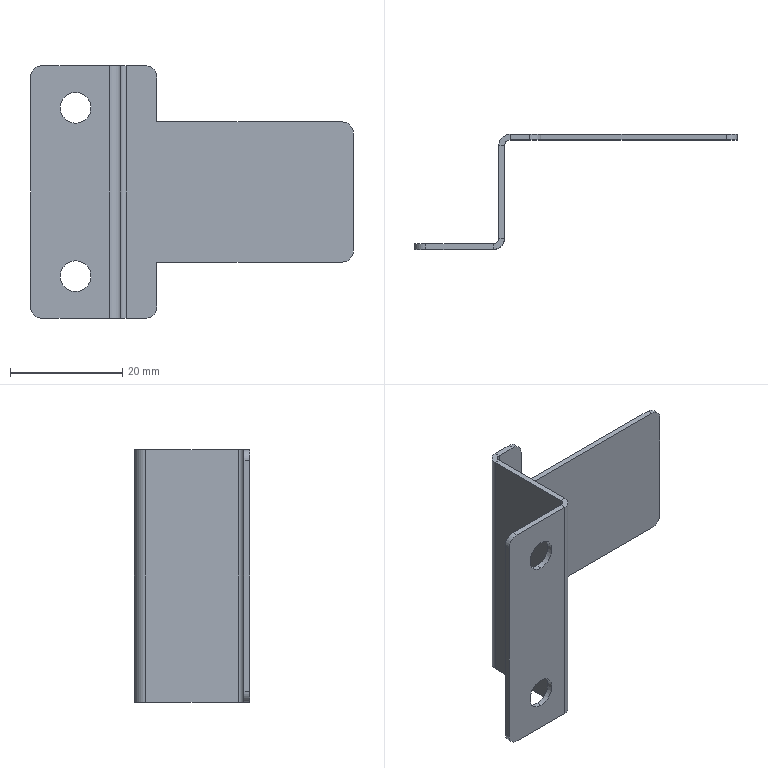Part | SolidWorks | features BaseBody 1 | 1 solid | 36 faces | box 57.5 x 20.5 x 45 mm | volume 2654 mm3 | plane 22 | cylinder 14 | commonest cylinder face diameters 4 x8 5.5 x4 2 x2
STEP:
#1=CARTESIAN_POINT('',(2.,-1.,45.));
#2=VERTEX_POINT('',#1);
#3=CARTESIAN_POINT('',(0.,-1.,43.));
#4=VERTEX_POINT('',#3);
#5=CARTESIAN_POINT('',(2.,-1.,43.));
#6=DIRECTION('',(0.,-1.,0.));
#7=DIRECTION('',(0.,0.,1.));
#8=AXIS2_PLACEMENT_3D('',#5,#6,#7);
#9=CIRCLE('',#8,2.);
#10=EDGE_CURVE('',#2,#4,#9,.T.);
#11=ORIENTED_EDGE('',*,*,#10,.F.);
#12=CARTESIAN_POINT('',(2.,0.,45.));
#13=VERTEX_POINT('',#12);
#14=CARTESIAN_POINT('',(2.,17.5,45.));
#15=DIRECTION('',(0.,-1.,0.));
#16=VECTOR('',#15,1000.);
#17=LINE('',#14,#16);
#18=EDGE_CURVE('',#13,#2,#17,.T.);
#19=ORIENTED_EDGE('',*,*,#18,.F.);
#20=CARTESIAN_POINT('',(0.,0.,43.));
#21=VERTEX_POINT('',#20);
#22=CARTESIAN_POINT('',(2.,0.,43.));
#23=DIRECTION('',(0.,1.,0.));
#24=DIRECTION('',(0.,0.,1.));
#25=AXIS2_PLACEMENT_3D('',#22,#23,#24);
#26=CIRCLE('',#25,2.);
#27=EDGE_CURVE('',#21,#13,#26,.T.);
#28=ORIENTED_EDGE('',*,*,#27,.F.);
#29=CARTESIAN_POINT('',(0.,-1.,43.));
#30=DIRECTION('',(0.,1.,0.));
#31=VECTOR('',#30,1000.);
#32=LINE('',#29,#31);
#33=EDGE_CURVE('',#4,#21,#32,.T.);
#34=ORIENTED_EDGE('',*,*,#33,.F.);
#35=EDGE_LOOP('',(#11,#19,#28,#34));
#36=FACE_OUTER_BOUND('',#35,.T.);
#37=CARTESIAN_POINT('',(2.,-1.,43.));
#38=DIRECTION('',(0.,1.,0.));
#39=DIRECTION('',(0.,0.,1.));
#40=AXIS2_PLACEMENT_3D('',#37,#38,#39);
#41=CYLINDRICAL_SURFACE('',#40,2.);
#42=ADVANCED_FACE('',(#36),#41,.T.);
#43=CARTESIAN_POINT('',(0.,-1.,2.));
#44=VERTEX_POINT('',#43);
#45=CARTESIAN_POINT('',(2.,-1.,0.));
#46=VERTEX_POINT('',#45);
#47=CARTESIAN_POINT('',(2.,-1.,2.));
#48=DIRECTION('',(0.,-1.,0.));
#49=DIRECTION('',(0.,0.,1.));
#50=AXIS2_PLACEMENT_3D('',#47,#48,#49);
#51=CIRCLE('',#50,2.);
#52=EDGE_CURVE('',#44,#46,#51,.T.);
#53=ORIENTED_EDGE('',*,*,#52,.F.);
#54=CARTESIAN_POINT('',(0.,0.,2.));
#55=VERTEX_POINT('',#54);
#56=CARTESIAN_POINT('',(0.,-1.,2.));
#57=DIRECTION('',(0.,-1.,0.));
#58=VECTOR('',#57,1000.);
#59=LINE('',#56,#58);
#60=EDGE_CURVE('',#55,#44,#59,.T.);
#61=ORIENTED_EDGE('',*,*,#60,.F.);
#62=CARTESIAN_POINT('',(2.,0.,0.));
#63=VERTEX_POINT('',#62);
#64=CARTESIAN_POINT('',(2.,0.,2.));
#65=DIRECTION('',(0.,1.,0.));
#66=DIRECTION('',(0.,0.,1.));
#67=AXIS2_PLACEMENT_3D('',#64,#65,#66);
#68=CIRCLE('',#67,2.);
#69=EDGE_CURVE('',#63,#55,#68,.T.);
#70=ORIENTED_EDGE('',*,*,#69,.F.);
#71=CARTESIAN_POINT('',(2.,1.,0.));
#72=DIRECTION('',(0.,1.,0.));
#73=VECTOR('',#72,1000.);
#74=LINE('',#71,#73);
#75=EDGE_CURVE('',#46,#63,#74,.T.);
#76=ORIENTED_EDGE('',*,*,#75,.F.);
#77=EDGE_LOOP('',(#53,#61,#70,#76));
#78=FACE_OUTER_BOUND('',#77,.T.);
#79=CARTESIAN_POINT('',(2.,1.,2.));
#80=DIRECTION('',(0.,1.,0.));
#81=DIRECTION('',(0.,0.,1.));
#82=AXIS2_PLACEMENT_3D('',#79,#80,#81);
#83=CYLINDRICAL_SURFACE('',#82,2.);
#84=ADVANCED_FACE('',(#78),#83,.T.);
#85=CARTESIAN_POINT('',(22.5,18.5,43.));
#86=VERTEX_POINT('',#85);
#87=CARTESIAN_POINT('',(20.5,18.5,45.));
#88=VERTEX_POINT('',#87);
#89=CARTESIAN_POINT('',(20.5,18.5,43.));
#90=DIRECTION('',(0.,-1.,0.));
#91=DIRECTION('',(0.,0.,1.));
#92=AXIS2_PLACEMENT_3D('',#89,#90,#91);
#93=CIRCLE('',#92,2.);
#94=EDGE_CURVE('',#86,#88,#93,.T.);
#95=ORIENTED_EDGE('',*,*,#94,.F.);
#96=CARTESIAN_POINT('',(22.5,19.5,43.));
#97=VERTEX_POINT('',#96);
#98=CARTESIAN_POINT('',(22.5,18.5,43.));
#99=DIRECTION('',(0.,-1.,0.));
#100=VECTOR('',#99,1000.);
#101=LINE('',#98,#100);
#102=EDGE_CURVE('',#97,#86,#101,.T.);
#103=ORIENTED_EDGE('',*,*,#102,.F.);
#104=CARTESIAN_POINT('',(20.5,19.5,45.));
#105=VERTEX_POINT('',#104);
#106=CARTESIAN_POINT('',(20.5,19.5,43.));
#107=DIRECTION('',(0.,1.,0.));
#108=DIRECTION('',(0.,0.,1.));
#109=AXIS2_PLACEMENT_3D('',#106,#107,#108);
#110=CIRCLE('',#109,2.);
#111=EDGE_CURVE('',#105,#97,#110,.T.);
#112=ORIENTED_EDGE('',*,*,#111,.F.);
#113=CARTESIAN_POINT('',(20.5,19.5,45.));
#114=DIRECTION('',(0.,1.,0.));
#115=VECTOR('',#114,1000.);
#116=LINE('',#113,#115);
#117=EDGE_CURVE('',#88,#105,#116,.T.);
#118=ORIENTED_EDGE('',*,*,#117,.F.);
#119=EDGE_LOOP('',(#95,#103,#112,#118));
#120=FACE_OUTER_BOUND('',#119,.T.);
#121=CARTESIAN_POINT('',(20.5,17.5,43.));
#122=DIRECTION('',(0.,-1.,0.));
#123=DIRECTION('',(0.,0.,-1.));
#124=AXIS2_PLACEMENT_3D('',#121,#122,#123);
#125=CYLINDRICAL_SURFACE('',#124,2.);
#126=ADVANCED_FACE('',(#120),#125,.T.);
#127=CARTESIAN_POINT('',(57.5,18.5,33.));
#128=VERTEX_POINT('',#127);
#129=CARTESIAN_POINT('',(55.5,18.5,35.));
#130=VERTEX_POINT('',#129);
#131=CARTESIAN_POINT('',(55.5,18.5,33.));
#132=DIRECTION('',(0.,-1.,0.));
#133=DIRECTION('',(0.,0.,1.));
#134=AXIS2_PLACEMENT_3D('',#131,#132,#133);
#135=CIRCLE('',#134,2.);
#136=EDGE_CURVE('',#128,#130,#135,.T.);
#137=ORIENTED_EDGE('',*,*,#136,.F.);
#138=CARTESIAN_POINT('',(57.5,19.5,33.));
#139=VERTEX_POINT('',#138);
#140=CARTESIAN_POINT('',(57.5,18.5,33.));
#141=DIRECTION('',(0.,-1.,0.));
#142=VECTOR('',#141,1000.);
#143=LINE('',#140,#142);
#144=EDGE_CURVE('',#139,#128,#143,.T.);
#145=ORIENTED_EDGE('',*,*,#144,.F.);
#146=CARTESIAN_POINT('',(55.5,19.5,35.));
#147=VERTEX_POINT('',#146);
#148=CARTESIAN_POINT('',(55.5,19.5,33.));
#149=DIRECTION('',(0.,1.,0.));
#150=DIRECTION('',(0.,0.,1.));
#151=AXIS2_PLACEMENT_3D('',#148,#149,#150);
#152=CIRCLE('',#151,2.);
#153=EDGE_CURVE('',#147,#139,#152,.T.);
#154=ORIENTED_EDGE('',*,*,#153,.F.);
#155=CARTESIAN_POINT('',(55.5,19.5,35.));
#156=DIRECTION('',(0.,1.,0.));
#157=VECTOR('',#156,1000.);
#158=LINE('',#155,#157);
#159=EDGE_CURVE('',#130,#147,#158,.T.);
#160=ORIENTED_EDGE('',*,*,#159,.F.);
#161=EDGE_LOOP('',(#137,#145,#154,#160));
#162=FACE_OUTER_BOUND('',#161,.T.);
#163=CARTESIAN_POINT('',(55.5,16.5,33.));
#164=DIRECTION('',(0.,-1.,0.));
#165=DIRECTION('',(0.,0.,-1.));
#166=AXIS2_PLACEMENT_3D('',#163,#164,#165);
#167=CYLINDRICAL_SURFACE('',#166,2.);
#168=ADVANCED_FACE('',(#162),#167,.T.);
#169=CARTESIAN_POINT('',(55.5,18.5,10.));
#170=VERTEX_POINT('',#169);
#171=CARTESIAN_POINT('',(57.5,18.5,12.));
#172=VERTEX_POINT('',#171);
#173=CARTESIAN_POINT('',(55.5,18.5,12.));
#174=DIRECTION('',(0.,-1.,0.));
#175=DIRECTION('',(0.,0.,1.));
#176=AXIS2_PLACEMENT_3D('',#173,#174,#175);
#177=CIRCLE('',#176,2.);
#178=EDGE_CURVE('',#170,#172,#177,.T.);
#179=ORIENTED_EDGE('',*,*,#178,.F.);
#180=CARTESIAN_POINT('',(55.5,19.5,10.));
#181=VERTEX_POINT('',#180);
#182=CARTESIAN_POINT('',(55.5,18.5,10.));
#183=DIRECTION('',(0.,-1.,0.));
#184=VECTOR('',#183,1000.);
#185=LINE('',#182,#184);
#186=EDGE_CURVE('',#181,#170,#185,.T.);
#187=ORIENTED_EDGE('',*,*,#186,.F.);
#188=CARTESIAN_POINT('',(57.5,19.5,12.));
#189=VERTEX_POINT('',#188);
#190=CARTESIAN_POINT('',(55.5,19.5,12.));
#191=DIRECTION('',(0.,1.,0.));
#192=DIRECTION('',(0.,0.,1.));
#193=AXIS2_PLACEMENT_3D('',#190,#191,#192);
#194=CIRCLE('',#193,2.);
#195=EDGE_CURVE('',#189,#181,#194,.T.);
#196=ORIENTED_EDGE('',*,*,#195,.F.);
#197=CARTESIAN_POINT('',(57.5,19.5,12.));
#198=DIRECTION('',(0.,1.,0.));
#199=VECTOR('',#198,1000.);
#200=LINE('',#197,#199);
#201=EDGE_CURVE('',#172,#189,#200,.T.);
#202=ORIENTED_EDGE('',*,*,#201,.F.);
#203=EDGE_LOOP('',(#179,#187,#196,#202));
#204=FACE_OUTER_BOUND('',#203,.T.);
#205=CARTESIAN_POINT('',(55.5,19.5,12.));
#206=DIRECTION('',(0.,-1.,0.));
#207=DIRECTION('',(0.,0.,-1.));
#208=AXIS2_PLACEMENT_3D('',#205,#206,#207);
#209=CYLINDRICAL_SURFACE('',#208,2.);
#210=ADVANCED_FACE('',(#204),#209,.T.);
#211=CARTESIAN_POINT('',(22.5,19.5,2.));
#212=VERTEX_POINT('',#211);
#213=CARTESIAN_POINT('',(20.5,19.5,0.));
#214=VERTEX_POINT('',#213);
#215=CARTESIAN_POINT('',(20.5,19.5,2.));
#216=DIRECTION('',(0.,1.,0.));
#217=DIRECTION('',(0.,0.,1.));
#218=AXIS2_PLACEMENT_3D('',#215,#216,#217);
#219=CIRCLE('',#218,2.);
#220=EDGE_CURVE('',#212,#214,#219,.T.);
#221=ORIENTED_EDGE('',*,*,#220,.F.);
#222=CARTESIAN_POINT('',(22.5,18.5,2.));
#223=VERTEX_POINT('',#222);
#224=CARTESIAN_POINT('',(22.5,16.5,2.));
#225=DIRECTION('',(0.,1.,0.));
#226=VECTOR('',#225,1000.);
#227=LINE('',#224,#226);
#228=EDGE_CURVE('',#223,#212,#227,.T.);
#229=ORIENTED_EDGE('',*,*,#228,.F.);
#230=CARTESIAN_POINT('',(20.5,18.5,0.));
#231=VERTEX_POINT('',#230);
#232=CARTESIAN_POINT('',(20.5,18.5,2.));
#233=DIRECTION('',(0.,-1.,0.));
#234=DIRECTION('',(0.,0.,1.));
#235=AXIS2_PLACEMENT_3D('',#232,#233,#234);
#236=CIRCLE('',#235,2.);
#237=EDGE_CURVE('',#231,#223,#236,.T.);
#238=ORIENTED_EDGE('',*,*,#237,.F.);
#239=CARTESIAN_POINT('',(20.5,17.5,0.));
#240=DIRECTION('',(0.,-1.,0.));
#241=VECTOR('',#240,1000.);
#242=LINE('',#239,#241);
#243=EDGE_CURVE('',#214,#231,#242,.T.);
#244=ORIENTED_EDGE('',*,*,#243,.F.);
#245=EDGE_LOOP('',(#221,#229,#238,#244));
#246=FACE_OUTER_BOUND('',#245,.T.);
#247=CARTESIAN_POINT('',(20.5,17.5,2.));
#248=DIRECTION('',(0.,-1.,0.));
#249=DIRECTION('',(0.,0.,-1.));
#250=AXIS2_PLACEMENT_3D('',#247,#248,#249);
#251=CYLINDRICAL_SURFACE('',#250,2.);
#252=ADVANCED_FACE('',(#246),#251,.T.);
#253=CARTESIAN_POINT('',(22.5,18.5,35.));
#254=VERTEX_POINT('',#253);
#255=CARTESIAN_POINT('',(15.,18.5,35.));
#256=DIRECTION('',(-1.,0.,0.));
#257=VECTOR('',#256,1000.);
#258=LINE('',#255,#257);
#259=EDGE_CURVE('',#130,#254,#258,.T.);
#260=ORIENTED_EDGE('',*,*,#259,.F.);
#261=ORIENTED_EDGE('',*,*,#159,.T.);
#262=CARTESIAN_POINT('',(22.5,19.5,35.));
#263=VERTEX_POINT('',#262);
#264=CARTESIAN_POINT('',(57.5,19.5,35.));
#265=DIRECTION('',(-1.,0.,0.));
#266=VECTOR('',#265,1000.);
#267=LINE('',#264,#266);
#268=EDGE_CURVE('',#147,#263,#267,.T.);
#269=ORIENTED_EDGE('',*,*,#268,.T.);
#270=CARTESIAN_POINT('',(22.5,16.5,35.));
#271=DIRECTION('',(0.,1.,0.));
#272=VECTOR('',#271,1000.);
#273=LINE('',#270,#272);
#274=EDGE_CURVE('',#254,#263,#273,.T.);
#275=ORIENTED_EDGE('',*,*,#274,.F.);
#276=EDGE_LOOP('',(#260,#261,#269,#275));
#277=FACE_OUTER_BOUND('',#276,.T.);
#278=CARTESIAN_POINT('',(57.5,16.5,35.));
#279=DIRECTION('',(0.,0.,-1.));
#280=DIRECTION('',(0.,-1.,0.));
#281=AXIS2_PLACEMENT_3D('',#278,#279,#280);
#282=PLANE('',#281);
#283=ADVANCED_FACE('',(#277),#282,.F.);
#284=CARTESIAN_POINT('',(22.5,19.5,45.));
#285=DIRECTION('',(0.,0.,1.));
#286=VECTOR('',#285,1000.);
#287=LINE('',#284,#286);
#288=EDGE_CURVE('',#263,#97,#287,.T.);
#289=ORIENTED_EDGE('',*,*,#288,.T.);
#290=ORIENTED_EDGE('',*,*,#102,.T.);
#291=CARTESIAN_POINT('',(22.5,18.5,45.));
#292=DIRECTION('',(0.,0.,1.));
#293=VECTOR('',#292,1000.);
#294=LINE('',#291,#293);
#295=EDGE_CURVE('',#254,#86,#294,.T.);
#296=ORIENTED_EDGE('',*,*,#295,.F.);
#297=ORIENTED_EDGE('',*,*,#274,.T.);
#298=EDGE_LOOP('',(#289,#290,#296,#297));
#299=FACE_OUTER_BOUND('',#298,.T.);
#300=CARTESIAN_POINT('',(22.5,16.5,45.));
#301=DIRECTION('',(-1.,0.,0.));
#302=DIRECTION('',(0.,0.,1.));
#303=AXIS2_PLACEMENT_3D('',#300,#301,#302);
#304=PLANE('',#303);
#305=ADVANCED_FACE('',(#299),#304,.F.);
#306=CARTESIAN_POINT('',(22.5,18.5,10.));
#307=VERTEX_POINT('',#306);
#308=CARTESIAN_POINT('',(22.5,18.5,45.));
#309=DIRECTION('',(0.,0.,1.));
#310=VECTOR('',#309,1000.);
#311=LINE('',#308,#310);
#312=EDGE_CURVE('',#223,#307,#311,.T.);
#313=ORIENTED_EDGE('',*,*,#312,.F.);
#314=ORIENTED_EDGE('',*,*,#228,.T.);
#315=CARTESIAN_POINT('',(22.5,19.5,10.));
#316=VERTEX_POINT('',#315);
#317=CARTESIAN_POINT('',(22.5,19.5,0.));
#318=DIRECTION('',(0.,0.,1.));
#319=VECTOR('',#318,1000.);
#320=LINE('',#317,#319);
#321=EDGE_CURVE('',#212,#316,#320,.T.);
#322=ORIENTED_EDGE('',*,*,#321,.T.);
#323=CARTESIAN_POINT('',(22.5,16.5,10.));
#324=DIRECTION('',(0.,1.,0.));
#325=VECTOR('',#324,1000.);
#326=LINE('',#323,#325);
#327=EDGE_CURVE('',#307,#316,#326,.T.);
#328=ORIENTED_EDGE('',*,*,#327,.F.);
#329=EDGE_LOOP('',(#313,#314,#322,#328));
#330=FACE_OUTER_BOUND('',#329,.T.);
#331=CARTESIAN_POINT('',(22.5,16.5,0.));
#332=DIRECTION('',(-1.,0.,0.));
#333=DIRECTION('',(0.,0.,1.));
#334=AXIS2_PLACEMENT_3D('',#331,#332,#333);
#335=PLANE('',#334);
#336=ADVANCED_FACE('',(#330),#335,.F.);
#337=CARTESIAN_POINT('',(57.5,19.5,10.));
#338=DIRECTION('',(1.,0.,0.));
#339=VECTOR('',#338,1000.);
#340=LINE('',#337,#339);
#341=EDGE_CURVE('',#316,#181,#340,.T.);
#342=ORIENTED_EDGE('',*,*,#341,.T.);
#343=ORIENTED_EDGE('',*,*,#186,.T.);
#344=CARTESIAN_POINT('',(15.,18.5,10.));
#345=DIRECTION('',(1.,0.,0.));
#346=VECTOR('',#345,1000.);
#347=LINE('',#344,#346);
#348=EDGE_CURVE('',#307,#170,#347,.T.);
#349=ORIENTED_EDGE('',*,*,#348,.F.);
#350=ORIENTED_EDGE('',*,*,#327,.T.);
#351=EDGE_LOOP('',(#342,#343,#349,#350));
#352=FACE_OUTER_BOUND('',#351,.T.);
#353=CARTESIAN_POINT('',(57.5,16.5,10.));
#354=DIRECTION('',(0.,0.,1.));
#355=DIRECTION('',(1.,0.,0.));
#356=AXIS2_PLACEMENT_3D('',#353,#354,#355);
#357=PLANE('',#356);
#358=ADVANCED_FACE('',(#352),#357,.F.);
#359=CARTESIAN_POINT('',(8.,-1.,4.75));
#360=VERTEX_POINT('',#359);
#361=CARTESIAN_POINT('',(8.,0.,4.75));
#362=VERTEX_POINT('',#361);
#363=CARTESIAN_POINT('',(8.,-8.778,4.75));
#364=DIRECTION('',(0.,1.,0.));
#365=VECTOR('',#364,1000.);
#366=LINE('',#363,#365);
#367=EDGE_CURVE('',#360,#362,#366,.T.);
#368=ORIENTED_EDGE('',*,*,#367,.F.);
#369=CARTESIAN_POINT('',(8.,-1.,10.25));
#370=VERTEX_POINT('',#369);
#371=CARTESIAN_POINT('',(8.,-1.,7.5));
#372=DIRECTION('',(0.,-1.,0.));
#373=DIRECTION('',(0.,0.,1.));
#374=AXIS2_PLACEMENT_3D('',#371,#372,#373);
#375=CIRCLE('',#374,2.75);
#376=EDGE_CURVE('',#360,#370,#375,.T.);
#377=ORIENTED_EDGE('',*,*,#376,.T.);
#378=CARTESIAN_POINT('',(8.,0.,10.25));
#379=VERTEX_POINT('',#378);
#380=CARTESIAN_POINT('',(8.,-8.778,10.25));
#381=DIRECTION('',(0.,1.,0.));
#382=VECTOR('',#381,1000.);
#383=LINE('',#380,#382);
#384=EDGE_CURVE('',#370,#379,#383,.T.);
#385=ORIENTED_EDGE('',*,*,#384,.T.);
#386=CARTESIAN_POINT('',(8.,0.,7.5));
#387=DIRECTION('',(0.,1.,0.));
#388=DIRECTION('',(0.,0.,1.));
#389=AXIS2_PLACEMENT_3D('',#386,#387,#388);
#390=CIRCLE('',#389,2.75);
#391=EDGE_CURVE('',#379,#362,#390,.T.);
#392=ORIENTED_EDGE('',*,*,#391,.T.);
#393=EDGE_LOOP('',(#368,#377,#385,#392));
#394=FACE_OUTER_BOUND('',#393,.T.);
#395=CARTESIAN_POINT('',(8.,-8.778,7.5));
#396=DIRECTION('',(0.,1.,0.));
#397=DIRECTION('',(0.,0.,1.));
#398=AXIS2_PLACEMENT_3D('',#395,#396,#397);
#399=CYLINDRICAL_SURFACE('',#398,2.75);
#400=ADVANCED_FACE('',(#394),#399,.F.);
#401=CARTESIAN_POINT('',(8.,-1.,34.75));
#402=VERTEX_POINT('',#401);
#403=CARTESIAN_POINT('',(8.,0.,34.75));
#404=VERTEX_POINT('',#403);
#405=CARTESIAN_POINT('',(8.,-8.778,34.75));
#406=DIRECTION('',(0.,1.,0.));
#407=VECTOR('',#406,1000.);
#408=LINE('',#405,#407);
#409=EDGE_CURVE('',#402,#404,#408,.T.);
#410=ORIENTED_EDGE('',*,*,#409,.F.);
#411=CARTESIAN_POINT('',(8.,-1.,40.25));
#412=VERTEX_POINT('',#411);
#413=CARTESIAN_POINT('',(8.,-1.,37.5));
#414=DIRECTION('',(0.,-1.,0.));
#415=DIRECTION('',(0.,0.,1.));
#416=AXIS2_PLACEMENT_3D('',#413,#414,#415);
#417=CIRCLE('',#416,2.75);
#418=EDGE_CURVE('',#402,#412,#417,.T.);
#419=ORIENTED_EDGE('',*,*,#418,.T.);
#420=CARTESIAN_POINT('',(8.,0.,40.25));
#421=VERTEX_POINT('',#420);
#422=CARTESIAN_POINT('',(8.,-8.778,40.25));
#423=DIRECTION('',(0.,1.,0.));
#424=VECTOR('',#423,1000.);
#425=LINE('',#422,#424);
#426=EDGE_CURVE('',#412,#421,#425,.T.);
#427=ORIENTED_EDGE('',*,*,#426,.T.);
#428=CARTESIAN_POINT('',(8.,0.,37.5));
#429=DIRECTION('',(0.,1.,0.));
#430=DIRECTION('',(0.,0.,1.));
#431=AXIS2_PLACEMENT_3D('',#428,#429,#430);
#432=CIRCLE('',#431,2.75);
#433=EDGE_CURVE('',#421,#404,#432,.T.);
#434=ORIENTED_EDGE('',*,*,#433,.T.);
#435=EDGE_LOOP('',(#410,#419,#427,#434));
#436=FACE_OUTER_BOUND('',#435,.T.);
#437=CARTESIAN_POINT('',(8.,-8.778,37.5));
#438=DIRECTION('',(0.,1.,0.));
#439=DIRECTION('',(0.,0.,1.));
#440=AXIS2_PLACEMENT_3D('',#437,#438,#439);
#441=CYLINDRICAL_SURFACE('',#440,2.75);
#442=ADVANCED_FACE('',(#436),#441,.F.);
#443=CARTESIAN_POINT('',(17.,19.5,0.));
#444=VERTEX_POINT('',#443);
#445=CARTESIAN_POINT('',(15.,19.5,0.));
#446=DIRECTION('',(1.,0.,0.));
#447=VECTOR('',#446,1000.);
#448=LINE('',#445,#447);
#449=EDGE_CURVE('',#444,#214,#448,.T.);
#450=ORIENTED_EDGE('',*,*,#449,.T.);
#451=ORIENTED_EDGE('',*,*,#243,.T.);
#452=CARTESIAN_POINT('',(17.,18.5,0.));
#453=VERTEX_POINT('',#452);
#454=CARTESIAN_POINT('',(15.,18.5,0.));
#455=DIRECTION('',(1.,0.,0.));
#456=VECTOR('',#455,1000.);
#457=LINE('',#454,#456);
#458=EDGE_CURVE('',#453,#231,#457,.T.);
#459=ORIENTED_EDGE('',*,*,#458,.F.);
#460=CARTESIAN_POINT('',(17.,18.5,0.));
#461=DIRECTION('',(0.,1.,0.));
#462=VECTOR('',#461,1000.);
#463=LINE('',#460,#462);
#464=EDGE_CURVE('',#453,#444,#463,.T.);
#465=ORIENTED_EDGE('',*,*,#464,.T.);
#466=EDGE_LOOP('',(#450,#451,#459,#465));
#467=FACE_OUTER_BOUND('',#466,.T.);
#468=CARTESIAN_POINT('',(17.,17.5,0.));
#469=DIRECTION('',(0.,0.,1.));
#470=DIRECTION('',(1.,0.,0.));
#471=AXIS2_PLACEMENT_3D('',#468,#469,#470);
#472=PLANE('',#471);
#473=ADVANCED_FACE('',(#467),#472,.F.);
#474=CARTESIAN_POINT('',(14.,0.,45.));
#475=VERTEX_POINT('',#474);
#476=CARTESIAN_POINT('',(0.,0.,45.));
#477=DIRECTION('',(1.,0.,0.));
#478=VECTOR('',#477,1000.);
#479=LINE('',#476,#478);
#480=EDGE_CURVE('',#13,#475,#479,.T.);
#481=ORIENTED_EDGE('',*,*,#480,.F.);
#482=ORIENTED_EDGE('',*,*,#18,.T.);
#483=CARTESIAN_POINT('',(14.,-1.,45.));
#484=VERTEX_POINT('',#483);
#485=CARTESIAN_POINT('',(0.,-1.,45.));
#486=DIRECTION('',(1.,0.,0.));
#487=VECTOR('',#486,1000.);
#488=LINE('',#485,#487);
#489=EDGE_CURVE('',#2,#484,#488,.T.);
#490=ORIENTED_EDGE('',*,*,#489,.T.);
#491=CARTESIAN_POINT('',(14.,-1.,45.));
#492=DIRECTION('',(0.,1.,0.));
#493=VECTOR('',#492,1000.);
#494=LINE('',#491,#493);
#495=EDGE_CURVE('',#484,#475,#494,.T.);
#496=ORIENTED_EDGE('',*,*,#495,.T.);
#497=EDGE_LOOP('',(#481,#482,#490,#496));
#498=FACE_OUTER_BOUND('',#497,.T.);
#499=CARTESIAN_POINT('',(17.,17.5,45.));
#500=DIRECTION('',(0.,0.,1.));
#501=DIRECTION('',(1.,0.,0.));
#502=AXIS2_PLACEMENT_3D('',#499,#500,#501);
#503=PLANE('',#502);
#504=ADVANCED_FACE('',(#498),#503,.T.);
#505=CARTESIAN_POINT('',(16.,17.5,0.));
#506=VERTEX_POINT('',#505);
#507=CARTESIAN_POINT('',(17.,17.5,0.));
#508=DIRECTION('',(0.,0.,-1.));
#509=DIRECTION('',(1.,0.,0.));
#510=AXIS2_PLACEMENT_3D('',#507,#508,#509);
#511=CIRCLE('',#510,1.);
#512=EDGE_CURVE('',#506,#453,#511,.T.);
#513=ORIENTED_EDGE('',*,*,#512,.T.);
#514=CARTESIAN_POINT('',(17.,18.5,45.));
#515=VERTEX_POINT('',#514);
#516=CARTESIAN_POINT('',(17.,18.5,45.));
#517=DIRECTION('',(0.,0.,-1.));
#518=VECTOR('',#517,1000.);
#519=LINE('',#516,#518);
#520=EDGE_CURVE('',#515,#453,#519,.T.);
#521=ORIENTED_EDGE('',*,*,#520,.F.);
#522=CARTESIAN_POINT('',(16.,17.5,45.));
#523=VERTEX_POINT('',#522);
#524=CARTESIAN_POINT('',(17.,17.5,45.));
#525=DIRECTION('',(0.,0.,-1.));
#526=DIRECTION('',(1.,0.,0.));
#527=AXIS2_PLACEMENT_3D('',#524,#525,#526);
#528=CIRCLE('',#527,1.);
#529=EDGE_CURVE('',#523,#515,#528,.T.);
#530=ORIENTED_EDGE('',*,*,#529,.F.);
#531=CARTESIAN_POINT('',(16.,17.5,45.));
#532=DIRECTION('',(0.,0.,-1.));
#533=VECTOR('',#532,1000.);
#534=LINE('',#531,#533);
#535=EDGE_CURVE('',#523,#506,#534,.T.);
#536=ORIENTED_EDGE('',*,*,#535,.T.);
#537=EDGE_LOOP('',(#513,#521,#530,#536));
#538=FACE_OUTER_BOUND('',#537,.T.);
#539=CARTESIAN_POINT('',(17.,17.5,45.));
#540=DIRECTION('',(0.,0.,-1.));
#541=DIRECTION('',(-1.,0.,0.));
#542=AXIS2_PLACEMENT_3D('',#539,#540,#541);
#543=CYLINDRICAL_SURFACE('',#542,1.);
#544=ADVANCED_FACE('',(#538),#543,.F.);
#545=CARTESIAN_POINT('',(16.,1.,0.));
#546=VERTEX_POINT('',#545);
#547=CARTESIAN_POINT('',(16.,0.,0.));
#548=DIRECTION('',(0.,1.,0.));
#549=VECTOR('',#548,1000.);
#550=LINE('',#547,#549);
#551=EDGE_CURVE('',#546,#506,#550,.T.);
#552=ORIENTED_EDGE('',*,*,#551,.T.);
#553=ORIENTED_EDGE('',*,*,#535,.F.);
#554=CARTESIAN_POINT('',(16.,1.,45.));
#555=VERTEX_POINT('',#554);
#556=CARTESIAN_POINT('',(16.,0.,45.));
#557=DIRECTION('',(0.,1.,0.));
#558=VECTOR('',#557,1000.);
#559=LINE('',#556,#558);
#560=EDGE_CURVE('',#555,#523,#559,.T.);
#561=ORIENTED_EDGE('',*,*,#560,.F.);
#562=CARTESIAN_POINT('',(16.,1.,45.));
#563=DIRECTION('',(0.,0.,-1.));
#564=VECTOR('',#563,1000.);
#565=LINE('',#562,#564);
#566=EDGE_CURVE('',#555,#546,#565,.T.);
#567=ORIENTED_EDGE('',*,*,#566,.T.);
#568=EDGE_LOOP('',(#552,#553,#561,#567));
#569=FACE_OUTER_BOUND('',#568,.T.);
#570=CARTESIAN_POINT('',(16.,0.,45.));
#571=DIRECTION('',(-1.,0.,0.));
#572=DIRECTION('',(0.,0.,1.));
#573=AXIS2_PLACEMENT_3D('',#570,#571,#572);
#574=PLANE('',#573);
#575=ADVANCED_FACE('',(#569),#574,.F.);
#576=CARTESIAN_POINT('',(14.,-1.,0.));
#577=VERTEX_POINT('',#576);
#578=CARTESIAN_POINT('',(14.,1.,0.));
#579=DIRECTION('',(0.,0.,1.));
#580=DIRECTION('',(1.,0.,0.));
#581=AXIS2_PLACEMENT_3D('',#578,#579,#580);
#582=CIRCLE('',#581,2.);
#583=EDGE_CURVE('',#577,#546,#582,.T.);
#584=ORIENTED_EDGE('',*,*,#583,.T.);
#585=ORIENTED_EDGE('',*,*,#566,.F.);
#586=CARTESIAN_POINT('',(14.,1.,45.));
#587=DIRECTION('',(0.,0.,1.));
#588=DIRECTION('',(1.,0.,0.));
#589=AXIS2_PLACEMENT_3D('',#586,#587,#588);
#590=CIRCLE('',#589,2.);
#591=EDGE_CURVE('',#484,#555,#590,.T.);
#592=ORIENTED_EDGE('',*,*,#591,.F.);
#593=CARTESIAN_POINT('',(14.,-1.,45.));
#594=DIRECTION('',(0.,0.,-1.));
#595=VECTOR('',#594,1000.);
#596=LINE('',#593,#595);
#597=EDGE_CURVE('',#484,#577,#596,.T.);
#598=ORIENTED_EDGE('',*,*,#597,.T.);
#599=EDGE_LOOP('',(#584,#585,#592,#598));
#600=FACE_OUTER_BOUND('',#599,.T.);
#601=CARTESIAN_POINT('',(14.,1.,45.));
#602=DIRECTION('',(0.,0.,-1.));
#603=DIRECTION('',(-1.,0.,0.));
#604=AXIS2_PLACEMENT_3D('',#601,#602,#603);
#605=CYLINDRICAL_SURFACE('',#604,2.);
#606=ADVANCED_FACE('',(#600),#605,.T.);
#607=CARTESIAN_POINT('',(8.,-1.,37.5));
#608=DIRECTION('',(0.,-1.,0.));
#609=DIRECTION('',(0.,0.,1.));
#610=AXIS2_PLACEMENT_3D('',#607,#608,#609);
#611=CIRCLE('',#610,2.75);
#612=EDGE_CURVE('',#412,#402,#611,.T.);
#613=ORIENTED_EDGE('',*,*,#612,.F.);
#614=ORIENTED_EDGE('',*,*,#418,.F.);
#615=EDGE_LOOP('',(#613,#614));
#616=FACE_BOUND('',#615,.T.);
#617=CARTESIAN_POINT('',(8.,-1.,7.5));
#618=DIRECTION('',(0.,-1.,0.));
#619=DIRECTION('',(0.,0.,1.));
#620=AXIS2_PLACEMENT_3D('',#617,#618,#619);
#621=CIRCLE('',#620,2.75);
#622=EDGE_CURVE('',#370,#360,#621,.T.);
#623=ORIENTED_EDGE('',*,*,#622,.F.);
#624=ORIENTED_EDGE('',*,*,#376,.F.);
#625=EDGE_LOOP('',(#623,#624));
#626=FACE_BOUND('',#625,.T.);
#627=CARTESIAN_POINT('',(0.,-1.,45.));
#628=DIRECTION('',(0.,0.,-1.));
#629=VECTOR('',#628,1000.);
#630=LINE('',#627,#629);
#631=EDGE_CURVE('',#4,#44,#630,.T.);
#632=ORIENTED_EDGE('',*,*,#631,.T.);
#633=ORIENTED_EDGE('',*,*,#52,.T.);
#634=CARTESIAN_POINT('',(0.,-1.,0.));
#635=DIRECTION('',(1.,0.,0.));
#636=VECTOR('',#635,1000.);
#637=LINE('',#634,#636);
#638=EDGE_CURVE('',#46,#577,#637,.T.);
#639=ORIENTED_EDGE('',*,*,#638,.T.);
#640=ORIENTED_EDGE('',*,*,#597,.F.);
#641=ORIENTED_EDGE('',*,*,#489,.F.);
#642=ORIENTED_EDGE('',*,*,#10,.T.);
#643=EDGE_LOOP('',(#632,#633,#639,#640,#641,#642));
#644=FACE_OUTER_BOUND('',#643,.T.);
#645=CARTESIAN_POINT('',(0.,-1.,45.));
#646=DIRECTION('',(0.,1.,0.));
#647=DIRECTION('',(1.,0.,0.));
#648=AXIS2_PLACEMENT_3D('',#645,#646,#647);
#649=PLANE('',#648);
#650=ADVANCED_FACE('',(#616,#626,#644),#649,.F.);
#651=CARTESIAN_POINT('',(0.,0.,45.));
#652=DIRECTION('',(0.,0.,-1.));
#653=VECTOR('',#652,1000.);
#654=LINE('',#651,#653);
#655=EDGE_CURVE('',#21,#55,#654,.T.);
#656=ORIENTED_EDGE('',*,*,#655,.T.);
#657=ORIENTED_EDGE('',*,*,#60,.T.);
#658=ORIENTED_EDGE('',*,*,#631,.F.);
#659=ORIENTED_EDGE('',*,*,#33,.T.);
#660=EDGE_LOOP('',(#656,#657,#658,#659));
#661=FACE_OUTER_BOUND('',#660,.T.);
#662=CARTESIAN_POINT('',(0.,-1.,45.));
#663=DIRECTION('',(-1.,0.,0.));
#664=DIRECTION('',(0.,0.,1.));
#665=AXIS2_PLACEMENT_3D('',#662,#663,#664);
#666=PLANE('',#665);
#667=ADVANCED_FACE('',(#661),#666,.T.);
#668=ORIENTED_EDGE('',*,*,#433,.F.);
#669=CARTESIAN_POINT('',(8.,0.,37.5));
#670=DIRECTION('',(0.,1.,0.));
#671=DIRECTION('',(0.,0.,1.));
#672=AXIS2_PLACEMENT_3D('',#669,#670,#671);
#673=CIRCLE('',#672,2.75);
#674=EDGE_CURVE('',#404,#421,#673,.T.);
#675=ORIENTED_EDGE('',*,*,#674,.F.);
#676=EDGE_LOOP('',(#668,#675));
#677=FACE_BOUND('',#676,.T.);
#678=ORIENTED_EDGE('',*,*,#391,.F.);
#679=CARTESIAN_POINT('',(8.,0.,7.5));
#680=DIRECTION('',(0.,1.,0.));
#681=DIRECTION('',(0.,0.,1.));
#682=AXIS2_PLACEMENT_3D('',#679,#680,#681);
#683=CIRCLE('',#682,2.75);
#684=EDGE_CURVE('',#362,#379,#683,.T.);
#685=ORIENTED_EDGE('',*,*,#684,.F.);
#686=EDGE_LOOP('',(#678,#685));
#687=FACE_BOUND('',#686,.T.);
#688=CARTESIAN_POINT('',(14.,0.,0.));
#689=VERTEX_POINT('',#688);
#690=CARTESIAN_POINT('',(0.,0.,0.));
#691=DIRECTION('',(1.,0.,0.));
#692=VECTOR('',#691,1000.);
#693=LINE('',#690,#692);
#694=EDGE_CURVE('',#63,#689,#693,.T.);
#695=ORIENTED_EDGE('',*,*,#694,.F.);
#696=ORIENTED_EDGE('',*,*,#69,.T.);
#697=ORIENTED_EDGE('',*,*,#655,.F.);
#698=ORIENTED_EDGE('',*,*,#27,.T.);
#699=ORIENTED_EDGE('',*,*,#480,.T.);
#700=CARTESIAN_POINT('',(14.,0.,45.));
#701=DIRECTION('',(0.,0.,-1.));
#702=VECTOR('',#701,1000.);
#703=LINE('',#700,#702);
#704=EDGE_CURVE('',#475,#689,#703,.T.);
#705=ORIENTED_EDGE('',*,*,#704,.T.);
#706=EDGE_LOOP('',(#695,#696,#697,#698,#699,#705));
#707=FACE_OUTER_BOUND('',#706,.T.);
#708=CARTESIAN_POINT('',(0.,0.,45.));
#709=DIRECTION('',(0.,1.,0.));
#710=DIRECTION('',(1.,0.,0.));
#711=AXIS2_PLACEMENT_3D('',#708,#709,#710);
#712=PLANE('',#711);
#713=ADVANCED_FACE('',(#677,#687,#707),#712,.T.);
#714=CARTESIAN_POINT('',(15.,1.,0.));
#715=VERTEX_POINT('',#714);
#716=CARTESIAN_POINT('',(14.,1.,0.));
#717=DIRECTION('',(0.,0.,1.));
#718=DIRECTION('',(-1.,0.,0.));
#719=AXIS2_PLACEMENT_3D('',#716,#717,#718);
#720=CIRCLE('',#719,1.);
#721=EDGE_CURVE('',#689,#715,#720,.T.);
#722=ORIENTED_EDGE('',*,*,#721,.F.);
#723=ORIENTED_EDGE('',*,*,#704,.F.);
#724=CARTESIAN_POINT('',(15.,1.,45.));
#725=VERTEX_POINT('',#724);
#726=CARTESIAN_POINT('',(14.,1.,45.));
#727=DIRECTION('',(0.,0.,1.));
#728=DIRECTION('',(-1.,0.,0.));
#729=AXIS2_PLACEMENT_3D('',#726,#727,#728);
#730=CIRCLE('',#729,1.);
#731=EDGE_CURVE('',#475,#725,#730,.T.);
#732=ORIENTED_EDGE('',*,*,#731,.T.);
#733=CARTESIAN_POINT('',(15.,1.,45.));
#734=DIRECTION('',(0.,0.,-1.));
#735=VECTOR('',#734,1000.);
#736=LINE('',#733,#735);
#737=EDGE_CURVE('',#725,#715,#736,.T.);
#738=ORIENTED_EDGE('',*,*,#737,.T.);
#739=EDGE_LOOP('',(#722,#723,#732,#738));
#740=FACE_OUTER_BOUND('',#739,.T.);
#741=CARTESIAN_POINT('',(14.,1.,45.));
#742=DIRECTION('',(0.,0.,-1.));
#743=DIRECTION('',(-1.,0.,0.));
#744=AXIS2_PLACEMENT_3D('',#741,#742,#743);
#745=CYLINDRICAL_SURFACE('',#744,1.);
#746=ADVANCED_FACE('',(#740),#745,.F.);
#747=CARTESIAN_POINT('',(15.,17.5,0.));
#748=VERTEX_POINT('',#747);
#749=CARTESIAN_POINT('',(15.,0.,0.));
#750=DIRECTION('',(0.,1.,0.));
#751=VECTOR('',#750,1000.);
#752=LINE('',#749,#751);
#753=EDGE_CURVE('',#715,#748,#752,.T.);
#754=ORIENTED_EDGE('',*,*,#753,.F.);
#755=ORIENTED_EDGE('',*,*,#737,.F.);
#756=CARTESIAN_POINT('',(15.,17.5,45.));
#757=VERTEX_POINT('',#756);
#758=CARTESIAN_POINT('',(15.,0.,45.));
#759=DIRECTION('',(0.,1.,0.));
#760=VECTOR('',#759,1000.);
#761=LINE('',#758,#760);
#762=EDGE_CURVE('',#725,#757,#761,.T.);
#763=ORIENTED_EDGE('',*,*,#762,.T.);
#764=CARTESIAN_POINT('',(15.,17.5,45.));
#765=DIRECTION('',(0.,0.,-1.));
#766=VECTOR('',#765,1000.);
#767=LINE('',#764,#766);
#768=EDGE_CURVE('',#757,#748,#767,.T.);
#769=ORIENTED_EDGE('',*,*,#768,.T.);
#770=EDGE_LOOP('',(#754,#755,#763,#769));
#771=FACE_OUTER_BOUND('',#770,.T.);
#772=CARTESIAN_POINT('',(15.,0.,45.));
#773=DIRECTION('',(-1.,0.,0.));
#774=DIRECTION('',(0.,0.,1.));
#775=AXIS2_PLACEMENT_3D('',#772,#773,#774);
#776=PLANE('',#775);
#777=ADVANCED_FACE('',(#771),#776,.T.);
#778=CARTESIAN_POINT('',(17.,17.5,0.));
#779=DIRECTION('',(0.,0.,-1.));
#780=DIRECTION('',(1.,0.,0.));
#781=AXIS2_PLACEMENT_3D('',#778,#779,#780);
#782=CIRCLE('',#781,2.);
#783=EDGE_CURVE('',#748,#444,#782,.T.);
#784=ORIENTED_EDGE('',*,*,#783,.F.);
#785=ORIENTED_EDGE('',*,*,#768,.F.);
#786=CARTESIAN_POINT('',(17.,19.5,45.));
#787=VERTEX_POINT('',#786);
#788=CARTESIAN_POINT('',(17.,17.5,45.));
#789=DIRECTION('',(0.,0.,-1.));
#790=DIRECTION('',(1.,0.,0.));
#791=AXIS2_PLACEMENT_3D('',#788,#789,#790);
#792=CIRCLE('',#791,2.);
#793=EDGE_CURVE('',#757,#787,#792,.T.);
#794=ORIENTED_EDGE('',*,*,#793,.T.);
#795=CARTESIAN_POINT('',(17.,19.5,45.));
#796=DIRECTION('',(0.,0.,-1.));
#797=VECTOR('',#796,1000.);
#798=LINE('',#795,#797);
#799=EDGE_CURVE('',#787,#444,#798,.T.);
#800=ORIENTED_EDGE('',*,*,#799,.T.);
#801=EDGE_LOOP('',(#784,#785,#794,#800));
#802=FACE_OUTER_BOUND('',#801,.T.);
#803=CARTESIAN_POINT('',(17.,17.5,45.));
#804=DIRECTION('',(0.,0.,-1.));
#805=DIRECTION('',(-1.,0.,0.));
#806=AXIS2_PLACEMENT_3D('',#803,#804,#805);
#807=CYLINDRICAL_SURFACE('',#806,2.);
#808=ADVANCED_FACE('',(#802),#807,.T.);
#809=ORIENTED_EDGE('',*,*,#321,.F.);
#810=ORIENTED_EDGE('',*,*,#220,.T.);
#811=ORIENTED_EDGE('',*,*,#449,.F.);
#812=ORIENTED_EDGE('',*,*,#799,.F.);
#813=CARTESIAN_POINT('',(15.,19.5,45.));
#814=DIRECTION('',(1.,0.,0.));
#815=VECTOR('',#814,1000.);
#816=LINE('',#813,#815);
#817=EDGE_CURVE('',#787,#105,#816,.T.);
#818=ORIENTED_EDGE('',*,*,#817,.T.);
#819=ORIENTED_EDGE('',*,*,#111,.T.);
#820=ORIENTED_EDGE('',*,*,#288,.F.);
#821=ORIENTED_EDGE('',*,*,#268,.F.);
#822=ORIENTED_EDGE('',*,*,#153,.T.);
#823=CARTESIAN_POINT('',(57.5,19.5,45.));
#824=DIRECTION('',(0.,0.,-1.));
#825=VECTOR('',#824,1000.);
#826=LINE('',#823,#825);
#827=EDGE_CURVE('',#139,#189,#826,.T.);
#828=ORIENTED_EDGE('',*,*,#827,.T.);
#829=ORIENTED_EDGE('',*,*,#195,.T.);
#830=ORIENTED_EDGE('',*,*,#341,.F.);
#831=EDGE_LOOP('',(#809,#810,#811,#812,#818,#819,#820,#821,#822,#828,#829,#830));
#832=FACE_OUTER_BOUND('',#831,.T.);
#833=CARTESIAN_POINT('',(15.,19.5,45.));
#834=DIRECTION('',(0.,1.,0.));
#835=DIRECTION('',(1.,0.,0.));
#836=AXIS2_PLACEMENT_3D('',#833,#834,#835);
#837=PLANE('',#836);
#838=ADVANCED_FACE('',(#832),#837,.T.);
#839=CARTESIAN_POINT('',(57.5,18.5,45.));
#840=DIRECTION('',(0.,0.,-1.));
#841=VECTOR('',#840,1000.);
#842=LINE('',#839,#841);
#843=EDGE_CURVE('',#128,#172,#842,.T.);
#844=ORIENTED_EDGE('',*,*,#843,.T.);
#845=ORIENTED_EDGE('',*,*,#201,.T.);
#846=ORIENTED_EDGE('',*,*,#827,.F.);
#847=ORIENTED_EDGE('',*,*,#144,.T.);
#848=EDGE_LOOP('',(#844,#845,#846,#847));
#849=FACE_OUTER_BOUND('',#848,.T.);
#850=CARTESIAN_POINT('',(57.5,19.5,45.));
#851=DIRECTION('',(1.,0.,0.));
#852=DIRECTION('',(0.,1.,0.));
#853=AXIS2_PLACEMENT_3D('',#850,#851,#852);
#854=PLANE('',#853);
#855=ADVANCED_FACE('',(#849),#854,.T.);
#856=ORIENTED_EDGE('',*,*,#458,.T.);
#857=ORIENTED_EDGE('',*,*,#237,.T.);
#858=ORIENTED_EDGE('',*,*,#312,.T.);
#859=ORIENTED_EDGE('',*,*,#348,.T.);
#860=ORIENTED_EDGE('',*,*,#178,.T.);
#861=ORIENTED_EDGE('',*,*,#843,.F.);
#862=ORIENTED_EDGE('',*,*,#136,.T.);
#863=ORIENTED_EDGE('',*,*,#259,.T.);
#864=ORIENTED_EDGE('',*,*,#295,.T.);
#865=ORIENTED_EDGE('',*,*,#94,.T.);
#866=CARTESIAN_POINT('',(15.,18.5,45.));
#867=DIRECTION('',(1.,0.,0.));
#868=VECTOR('',#867,1000.);
#869=LINE('',#866,#868);
#870=EDGE_CURVE('',#515,#88,#869,.T.);
#871=ORIENTED_EDGE('',*,*,#870,.F.);
#872=ORIENTED_EDGE('',*,*,#520,.T.);
#873=EDGE_LOOP('',(#856,#857,#858,#859,#860,#861,#862,#863,#864,#865,#871,#872));
#874=FACE_OUTER_BOUND('',#873,.T.);
#875=CARTESIAN_POINT('',(15.,18.5,45.));
#876=DIRECTION('',(0.,1.,0.));
#877=DIRECTION('',(1.,0.,0.));
#878=AXIS2_PLACEMENT_3D('',#875,#876,#877);
#879=PLANE('',#878);
#880=ADVANCED_FACE('',(#874),#879,.F.);
#881=ORIENTED_EDGE('',*,*,#753,.T.);
#882=CARTESIAN_POINT('',(15.,17.5,0.));
#883=DIRECTION('',(1.,0.,0.));
#884=VECTOR('',#883,1000.);
#885=LINE('',#882,#884);
#886=EDGE_CURVE('',#748,#506,#885,.T.);
#887=ORIENTED_EDGE('',*,*,#886,.T.);
#888=ORIENTED_EDGE('',*,*,#551,.F.);
#889=CARTESIAN_POINT('',(16.,1.,0.));
#890=DIRECTION('',(-1.,0.,0.));
#891=VECTOR('',#890,1000.);
#892=LINE('',#889,#891);
#893=EDGE_CURVE('',#546,#715,#892,.T.);
#894=ORIENTED_EDGE('',*,*,#893,.T.);
#895=EDGE_LOOP('',(#881,#887,#888,#894));
#896=FACE_OUTER_BOUND('',#895,.T.);
#897=CARTESIAN_POINT('',(17.,18.5,0.));
#898=DIRECTION('',(0.,0.,-1.));
#899=DIRECTION('',(0.,-1.,0.));
#900=AXIS2_PLACEMENT_3D('',#897,#898,#899);
#901=PLANE('',#900);
#902=ADVANCED_FACE('',(#896),#901,.T.);
#903=ORIENTED_EDGE('',*,*,#886,.F.);
#904=ORIENTED_EDGE('',*,*,#783,.T.);
#905=ORIENTED_EDGE('',*,*,#464,.F.);
#906=ORIENTED_EDGE('',*,*,#512,.F.);
#907=EDGE_LOOP('',(#903,#904,#905,#906));
#908=FACE_OUTER_BOUND('',#907,.T.);
#909=CARTESIAN_POINT('',(15.,17.5,0.));
#910=DIRECTION('',(0.,0.,-1.));
#911=DIRECTION('',(0.,-1.,0.));
#912=AXIS2_PLACEMENT_3D('',#909,#910,#911);
#913=PLANE('',#912);
#914=ADVANCED_FACE('',(#908),#913,.T.);
#915=ORIENTED_EDGE('',*,*,#870,.T.);
#916=ORIENTED_EDGE('',*,*,#117,.T.);
#917=ORIENTED_EDGE('',*,*,#817,.F.);
#918=CARTESIAN_POINT('',(17.,19.5,45.));
#919=DIRECTION('',(0.,-1.,0.));
#920=VECTOR('',#919,1000.);
#921=LINE('',#918,#920);
#922=EDGE_CURVE('',#787,#515,#921,.T.);
#923=ORIENTED_EDGE('',*,*,#922,.T.);
#924=EDGE_LOOP('',(#915,#916,#917,#923));
#925=FACE_OUTER_BOUND('',#924,.T.);
#926=CARTESIAN_POINT('',(16.,17.5,45.));
#927=DIRECTION('',(0.,0.,1.));
#928=DIRECTION('',(1.,0.,0.));
#929=AXIS2_PLACEMENT_3D('',#926,#927,#928);
#930=PLANE('',#929);
#931=ADVANCED_FACE('',(#925),#930,.T.);
#932=ORIENTED_EDGE('',*,*,#922,.F.);
#933=ORIENTED_EDGE('',*,*,#793,.F.);
#934=CARTESIAN_POINT('',(16.,17.5,45.));
#935=DIRECTION('',(-1.,0.,0.));
#936=VECTOR('',#935,1000.);
#937=LINE('',#934,#936);
#938=EDGE_CURVE('',#523,#757,#937,.T.);
#939=ORIENTED_EDGE('',*,*,#938,.F.);
#940=ORIENTED_EDGE('',*,*,#529,.T.);
#941=EDGE_LOOP('',(#932,#933,#939,#940));
#942=FACE_OUTER_BOUND('',#941,.T.);
#943=CARTESIAN_POINT('',(17.,19.5,45.));
#944=DIRECTION('',(0.,0.,1.));
#945=DIRECTION('',(1.,0.,0.));
#946=AXIS2_PLACEMENT_3D('',#943,#944,#945);
#947=PLANE('',#946);
#948=ADVANCED_FACE('',(#942),#947,.T.);
#949=ORIENTED_EDGE('',*,*,#638,.F.);
#950=ORIENTED_EDGE('',*,*,#75,.T.);
#951=ORIENTED_EDGE('',*,*,#694,.T.);
#952=CARTESIAN_POINT('',(14.,0.,0.));
#953=DIRECTION('',(0.,-1.,0.));
#954=VECTOR('',#953,1000.);
#955=LINE('',#952,#954);
#956=EDGE_CURVE('',#689,#577,#955,.T.);
#957=ORIENTED_EDGE('',*,*,#956,.T.);
#958=EDGE_LOOP('',(#949,#950,#951,#957));
#959=FACE_OUTER_BOUND('',#958,.T.);
#960=CARTESIAN_POINT('',(16.,1.,0.));
#961=DIRECTION('',(0.,0.,-1.));
#962=DIRECTION('',(0.,-1.,0.));
#963=AXIS2_PLACEMENT_3D('',#960,#961,#962);
#964=PLANE('',#963);
#965=ADVANCED_FACE('',(#959),#964,.T.);
#966=ORIENTED_EDGE('',*,*,#956,.F.);
#967=ORIENTED_EDGE('',*,*,#721,.T.);
#968=ORIENTED_EDGE('',*,*,#893,.F.);
#969=ORIENTED_EDGE('',*,*,#583,.F.);
#970=EDGE_LOOP('',(#966,#967,#968,#969));
#971=FACE_OUTER_BOUND('',#970,.T.);
#972=CARTESIAN_POINT('',(14.,0.,0.));
#973=DIRECTION('',(0.,0.,-1.));
#974=DIRECTION('',(0.,-1.,0.));
#975=AXIS2_PLACEMENT_3D('',#972,#973,#974);
#976=PLANE('',#975);
#977=ADVANCED_FACE('',(#971),#976,.T.);
#978=ORIENTED_EDGE('',*,*,#762,.F.);
#979=CARTESIAN_POINT('',(15.,1.,45.));
#980=DIRECTION('',(1.,0.,0.));
#981=VECTOR('',#980,1000.);
#982=LINE('',#979,#981);
#983=EDGE_CURVE('',#725,#555,#982,.T.);
#984=ORIENTED_EDGE('',*,*,#983,.T.);
#985=ORIENTED_EDGE('',*,*,#560,.T.);
#986=ORIENTED_EDGE('',*,*,#938,.T.);
#987=EDGE_LOOP('',(#978,#984,#985,#986));
#988=FACE_OUTER_BOUND('',#987,.T.);
#989=CARTESIAN_POINT('',(14.,-1.,45.));
#990=DIRECTION('',(0.,0.,1.));
#991=DIRECTION('',(1.,0.,0.));
#992=AXIS2_PLACEMENT_3D('',#989,#990,#991);
#993=PLANE('',#992);
#994=ADVANCED_FACE('',(#988),#993,.T.);
#995=ORIENTED_EDGE('',*,*,#983,.F.);
#996=ORIENTED_EDGE('',*,*,#731,.F.);
#997=ORIENTED_EDGE('',*,*,#495,.F.);
#998=ORIENTED_EDGE('',*,*,#591,.T.);
#999=EDGE_LOOP('',(#995,#996,#997,#998));
#1000=FACE_OUTER_BOUND('',#999,.T.);
#1001=CARTESIAN_POINT('',(15.,1.,45.));
#1002=DIRECTION('',(0.,0.,1.));
#1003=DIRECTION('',(1.,0.,0.));
#1004=AXIS2_PLACEMENT_3D('',#1001,#1002,#1003);
#1005=PLANE('',#1004);
#1006=ADVANCED_FACE('',(#1000),#1005,.T.);
#1007=ORIENTED_EDGE('',*,*,#612,.T.);
#1008=ORIENTED_EDGE('',*,*,#409,.T.);
#1009=ORIENTED_EDGE('',*,*,#674,.T.);
#1010=ORIENTED_EDGE('',*,*,#426,.F.);
#1011=EDGE_LOOP('',(#1007,#1008,#1009,#1010));
#1012=FACE_OUTER_BOUND('',#1011,.T.);
#1013=CARTESIAN_POINT('',(8.,-8.778,37.5));
#1014=DIRECTION('',(0.,1.,0.));
#1015=DIRECTION('',(0.,0.,1.));
#1016=AXIS2_PLACEMENT_3D('',#1013,#1014,#1015);
#1017=CYLINDRICAL_SURFACE('',#1016,2.75);
#1018=ADVANCED_FACE('',(#1012),#1017,.F.);
#1019=ORIENTED_EDGE('',*,*,#622,.T.);
#1020=ORIENTED_EDGE('',*,*,#367,.T.);
#1021=ORIENTED_EDGE('',*,*,#684,.T.);
#1022=ORIENTED_EDGE('',*,*,#384,.F.);
#1023=EDGE_LOOP('',(#1019,#1020,#1021,#1022));
#1024=FACE_OUTER_BOUND('',#1023,.T.);
#1025=CARTESIAN_POINT('',(8.,-8.778,7.5));
#1026=DIRECTION('',(0.,1.,0.));
#1027=DIRECTION('',(0.,0.,1.));
#1028=AXIS2_PLACEMENT_3D('',#1025,#1026,#1027);
#1029=CYLINDRICAL_SURFACE('',#1028,2.75);
#1030=ADVANCED_FACE('',(#1024),#1029,.F.);
#1031=CLOSED_SHELL('',(#42,#84,#126,#168,#210,#252,#283,#305,#336,#358,#400,#442,#473,#504,#544,#575,#606,#650,#667,#713,#746,#777,#808,#838,#855,#880,#902,#914,#931,#948,#965,#977,#994,#1006,#1018,#1030));
#1032=MANIFOLD_SOLID_BREP('',#1031);
#1033=CARTESIAN_POINT('',(0.,0.,0.));
#1034=DIRECTION('',(0.,0.,1.));
#1035=DIRECTION('',(1.,0.,0.));
#1036=AXIS2_PLACEMENT_3D('',#1033,#1034,#1035);
#1037=(LENGTH_UNIT()NAMED_UNIT(*)SI_UNIT(.MILLI.,.METRE.));
#1038=UNCERTAINTY_MEASURE_WITH_UNIT(LENGTH_MEASURE(0.00001),#1037,'','');
#1039=(NAMED_UNIT(*)PLANE_ANGLE_UNIT()SI_UNIT($,.RADIAN.));
#1040=(NAMED_UNIT(*)SI_UNIT($,.STERADIAN.)SOLID_ANGLE_UNIT());
#1041=(GEOMETRIC_REPRESENTATION_CONTEXT(3)GLOBAL_UNCERTAINTY_ASSIGNED_CONTEXT((#1038))GLOBAL_UNIT_ASSIGNED_CONTEXT((#1037,#1039,#1040))REPRESENTATION_CONTEXT('',''));
#1042=ADVANCED_BREP_SHAPE_REPRESENTATION('',(#1032,#1036),#1041);